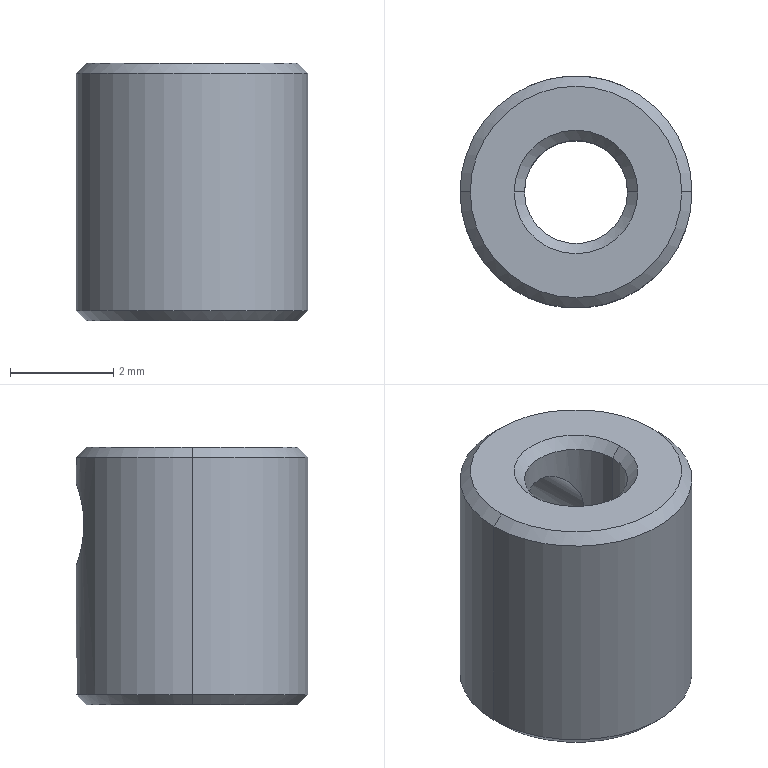Part | SolidWorks | features Chamfer 1, Extrusion 1, HoleWzd 1 | 1 solid | 16 faces | box 4.5 x 4.5 x 5 mm | volume 60.379 mm3 | cone 8 | cylinder 6 | plane 2 | commonest cylinder face diameters 1.6 x2 2 x2 4.5 x2
STEP:
#1=CARTESIAN_POINT('',(0.,2.25,1.8));
#2=VERTEX_POINT('',#1);
#3=CARTESIAN_POINT('',(0.,2.25,0.2));
#4=VERTEX_POINT('',#3);
#5=CARTESIAN_POINT('',(0.,2.25,1.8));
#6=CARTESIAN_POINT('',(-0.105,2.25,1.8));
#7=CARTESIAN_POINT('',(-0.211,2.242,1.779));
#8=CARTESIAN_POINT('',(-0.4042,2.216,1.698));
#9=CARTESIAN_POINT('',(-0.492,2.197,1.639));
#10=CARTESIAN_POINT('',(-0.6398,2.158,1.491));
#11=CARTESIAN_POINT('',(-0.6983,2.139,1.404));
#12=CARTESIAN_POINT('',(-0.779,2.111,1.21));
#13=CARTESIAN_POINT('',(-0.8,2.103,1.105));
#14=CARTESIAN_POINT('',(-0.8,2.103,0.8943));
#15=CARTESIAN_POINT('',(-0.7786,2.111,0.7885));
#16=CARTESIAN_POINT('',(-0.6983,2.139,0.5959));
#17=CARTESIAN_POINT('',(-0.639,2.159,0.5076));
#18=CARTESIAN_POINT('',(-0.4923,2.197,0.361));
#19=CARTESIAN_POINT('',(-0.4046,2.215,0.3019));
#20=CARTESIAN_POINT('',(-0.2107,2.242,0.2211));
#21=CARTESIAN_POINT('',(-0.1066,2.25,0.2));
#22=CARTESIAN_POINT('',(0.,2.25,0.2));
#23=B_SPLINE_CURVE_WITH_KNOTS('',3,(#5,#6,#7,#8,#9,#10,#11,#12,#13,#14,#15,#16,#17,#18,#19,#20,#21,#22),.UNSPECIFIED.,.F.,.F.,(4,2,2,2,2,2,2,2,4),(0.002522,0.002837,0.003152,0.003467,0.003783,0.004098,0.004413,0.004728,0.005043),.UNSPECIFIED.);
#24=EDGE_CURVE('',#2,#4,#23,.T.);
#25=ORIENTED_EDGE('',*,*,#24,.F.);
#26=CARTESIAN_POINT('',(0.,1.,1.8));
#27=VERTEX_POINT('',#26);
#28=CARTESIAN_POINT('',(0.,0.,1.8));
#29=DIRECTION('',(0.,-1.,0.));
#30=VECTOR('',#29,1000.);
#31=LINE('',#28,#30);
#32=EDGE_CURVE('',#2,#27,#31,.T.);
#33=ORIENTED_EDGE('',*,*,#32,.T.);
#34=CARTESIAN_POINT('',(0.,1.,0.2));
#35=VERTEX_POINT('',#34);
#36=CARTESIAN_POINT('',(0.,1.,1.8));
#37=CARTESIAN_POINT('',(-0.1101,1.,1.8));
#38=CARTESIAN_POINT('',(-0.2209,0.9807,1.776));
#39=CARTESIAN_POINT('',(-0.4161,0.9151,1.692));
#40=CARTESIAN_POINT('',(-0.5007,0.8698,1.632));
#41=CARTESIAN_POINT('',(-0.6401,0.7729,1.49));
#42=CARTESIAN_POINT('',(-0.6961,0.7204,1.407));
#43=CARTESIAN_POINT('',(-0.7755,0.6341,1.221));
#44=CARTESIAN_POINT('',(-0.7999,0.6001,1.112));
#45=CARTESIAN_POINT('',(-0.8001,0.5999,0.8891));
#46=CARTESIAN_POINT('',(-0.7764,0.6331,0.7814));
#47=CARTESIAN_POINT('',(-0.6962,0.7203,0.5928));
#48=CARTESIAN_POINT('',(-0.641,0.7723,0.511));
#49=CARTESIAN_POINT('',(-0.5007,0.8698,0.3681));
#50=CARTESIAN_POINT('',(-0.4177,0.9144,0.3094));
#51=CARTESIAN_POINT('',(-0.2225,0.9804,0.2242));
#52=CARTESIAN_POINT('',(-0.1119,1.,0.2));
#53=CARTESIAN_POINT('',(0.,1.,0.2));
#54=B_SPLINE_CURVE_WITH_KNOTS('',3,(#36,#37,#38,#39,#40,#41,#42,#43,#44,#45,#46,#47,#48,#49,#50,#51,#52,#53),.UNSPECIFIED.,.F.,.F.,(4,2,2,2,2,2,2,2,4),(0.002649,0.002979,0.003309,0.003639,0.003969,0.004299,0.00463,0.00496,0.00529),.UNSPECIFIED.);
#55=EDGE_CURVE('',#27,#35,#54,.T.);
#56=ORIENTED_EDGE('',*,*,#55,.T.);
#57=CARTESIAN_POINT('',(0.,0.,0.2));
#58=DIRECTION('',(0.,-1.,0.));
#59=VECTOR('',#58,1000.);
#60=LINE('',#57,#59);
#61=EDGE_CURVE('',#4,#35,#60,.T.);
#62=ORIENTED_EDGE('',*,*,#61,.F.);
#63=EDGE_LOOP('',(#25,#33,#56,#62));
#64=FACE_OUTER_BOUND('',#63,.T.);
#65=CARTESIAN_POINT('',(0.,0.,1.));
#66=DIRECTION('',(0.,-1.,0.));
#67=DIRECTION('',(0.,0.,-1.));
#68=AXIS2_PLACEMENT_3D('',#65,#66,#67);
#69=CYLINDRICAL_SURFACE('',#68,0.8);
#70=ADVANCED_FACE('',(#64),#69,.F.);
#71=CARTESIAN_POINT('',(2.05,0.,2.5));
#72=VERTEX_POINT('',#71);
#73=CARTESIAN_POINT('',(-2.05,0.,2.5));
#74=VERTEX_POINT('',#73);
#75=CARTESIAN_POINT('',(0.,0.,2.5));
#76=DIRECTION('',(0.,0.,1.));
#77=DIRECTION('',(1.,0.,0.));
#78=AXIS2_PLACEMENT_3D('',#75,#76,#77);
#79=CIRCLE('',#78,2.05);
#80=EDGE_CURVE('',#72,#74,#79,.T.);
#81=ORIENTED_EDGE('',*,*,#80,.F.);
#82=CARTESIAN_POINT('',(2.25,0.,2.3));
#83=VERTEX_POINT('',#82);
#84=CARTESIAN_POINT('',(2.05,0.,2.5));
#85=DIRECTION('',(0.7071,0.,-0.7071));
#86=VECTOR('',#85,1000.);
#87=LINE('',#84,#86);
#88=EDGE_CURVE('',#72,#83,#87,.T.);
#89=ORIENTED_EDGE('',*,*,#88,.T.);
#90=CARTESIAN_POINT('',(-2.25,0.,2.3));
#91=VERTEX_POINT('',#90);
#92=CARTESIAN_POINT('',(0.,0.,2.3));
#93=DIRECTION('',(0.,0.,-1.));
#94=DIRECTION('',(1.,0.,0.));
#95=AXIS2_PLACEMENT_3D('',#92,#93,#94);
#96=CIRCLE('',#95,2.25);
#97=EDGE_CURVE('',#91,#83,#96,.T.);
#98=ORIENTED_EDGE('',*,*,#97,.F.);
#99=CARTESIAN_POINT('',(-2.05,0.,2.5));
#100=DIRECTION('',(-0.7071,0.,-0.7071));
#101=VECTOR('',#100,1000.);
#102=LINE('',#99,#101);
#103=EDGE_CURVE('',#74,#91,#102,.T.);
#104=ORIENTED_EDGE('',*,*,#103,.F.);
#105=EDGE_LOOP('',(#81,#89,#98,#104));
#106=FACE_OUTER_BOUND('',#105,.T.);
#107=CARTESIAN_POINT('',(0.,0.,2.5));
#108=DIRECTION('',(0.,0.,-1.));
#109=DIRECTION('',(-1.,0.,0.));
#110=AXIS2_PLACEMENT_3D('',#107,#108,#109);
#111=CONICAL_SURFACE('',#110,2.05,0.7854);
#112=ADVANCED_FACE('',(#106),#111,.T.);
#113=CARTESIAN_POINT('',(-2.05,0.,-2.5));
#114=VERTEX_POINT('',#113);
#115=CARTESIAN_POINT('',(2.05,0.,-2.5));
#116=VERTEX_POINT('',#115);
#117=CARTESIAN_POINT('',(0.,0.,-2.5));
#118=DIRECTION('',(0.,0.,-1.));
#119=DIRECTION('',(1.,0.,0.));
#120=AXIS2_PLACEMENT_3D('',#117,#118,#119);
#121=CIRCLE('',#120,2.05);
#122=EDGE_CURVE('',#114,#116,#121,.T.);
#123=ORIENTED_EDGE('',*,*,#122,.F.);
#124=CARTESIAN_POINT('',(-2.25,0.,-2.3));
#125=VERTEX_POINT('',#124);
#126=CARTESIAN_POINT('',(-2.25,0.,-2.3));
#127=DIRECTION('',(-0.7071,0.,0.7071));
#128=VECTOR('',#127,1000.);
#129=LINE('',#126,#128);
#130=EDGE_CURVE('',#114,#125,#129,.T.);
#131=ORIENTED_EDGE('',*,*,#130,.T.);
#132=CARTESIAN_POINT('',(2.25,0.,-2.3));
#133=VERTEX_POINT('',#132);
#134=CARTESIAN_POINT('',(0.,0.,-2.3));
#135=DIRECTION('',(0.,0.,1.));
#136=DIRECTION('',(1.,0.,0.));
#137=AXIS2_PLACEMENT_3D('',#134,#135,#136);
#138=CIRCLE('',#137,2.25);
#139=EDGE_CURVE('',#133,#125,#138,.T.);
#140=ORIENTED_EDGE('',*,*,#139,.F.);
#141=CARTESIAN_POINT('',(2.25,0.,-2.3));
#142=DIRECTION('',(0.7071,0.,0.7071));
#143=VECTOR('',#142,1000.);
#144=LINE('',#141,#143);
#145=EDGE_CURVE('',#116,#133,#144,.T.);
#146=ORIENTED_EDGE('',*,*,#145,.F.);
#147=EDGE_LOOP('',(#123,#131,#140,#146));
#148=FACE_OUTER_BOUND('',#147,.T.);
#149=CARTESIAN_POINT('',(0.,0.,-2.3));
#150=DIRECTION('',(0.,0.,1.));
#151=DIRECTION('',(1.,0.,0.));
#152=AXIS2_PLACEMENT_3D('',#149,#150,#151);
#153=CONICAL_SURFACE('',#152,2.25,0.7854);
#154=ADVANCED_FACE('',(#148),#153,.T.);
#155=CARTESIAN_POINT('',(-1.,0.,2.3));
#156=VERTEX_POINT('',#155);
#157=CARTESIAN_POINT('',(1.,0.,2.3));
#158=VERTEX_POINT('',#157);
#159=CARTESIAN_POINT('',(0.,0.,2.3));
#160=DIRECTION('',(0.,0.,1.));
#161=DIRECTION('',(1.,0.,0.));
#162=AXIS2_PLACEMENT_3D('',#159,#160,#161);
#163=CIRCLE('',#162,1.);
#164=EDGE_CURVE('',#156,#158,#163,.T.);
#165=ORIENTED_EDGE('',*,*,#164,.F.);
#166=CARTESIAN_POINT('',(-1.2,0.,2.5));
#167=VERTEX_POINT('',#166);
#168=CARTESIAN_POINT('',(-1.,0.,2.3));
#169=DIRECTION('',(-0.7071,0.,0.7071));
#170=VECTOR('',#169,1000.);
#171=LINE('',#168,#170);
#172=EDGE_CURVE('',#156,#167,#171,.T.);
#173=ORIENTED_EDGE('',*,*,#172,.T.);
#174=CARTESIAN_POINT('',(1.2,0.,2.5));
#175=VERTEX_POINT('',#174);
#176=CARTESIAN_POINT('',(0.,0.,2.5));
#177=DIRECTION('',(0.,0.,-1.));
#178=DIRECTION('',(1.,0.,0.));
#179=AXIS2_PLACEMENT_3D('',#176,#177,#178);
#180=CIRCLE('',#179,1.2);
#181=EDGE_CURVE('',#175,#167,#180,.T.);
#182=ORIENTED_EDGE('',*,*,#181,.F.);
#183=CARTESIAN_POINT('',(1.,0.,2.3));
#184=DIRECTION('',(0.7071,0.,0.7071));
#185=VECTOR('',#184,1000.);
#186=LINE('',#183,#185);
#187=EDGE_CURVE('',#158,#175,#186,.T.);
#188=ORIENTED_EDGE('',*,*,#187,.F.);
#189=EDGE_LOOP('',(#165,#173,#182,#188));
#190=FACE_OUTER_BOUND('',#189,.T.);
#191=CARTESIAN_POINT('',(0.,0.,2.3));
#192=DIRECTION('',(0.,0.,1.));
#193=DIRECTION('',(1.,0.,0.));
#194=AXIS2_PLACEMENT_3D('',#191,#192,#193);
#195=CONICAL_SURFACE('',#194,1.,0.7854);
#196=ADVANCED_FACE('',(#190),#195,.F.);
#197=CARTESIAN_POINT('',(1.,0.,-2.3));
#198=VERTEX_POINT('',#197);
#199=CARTESIAN_POINT('',(-1.,0.,-2.3));
#200=VERTEX_POINT('',#199);
#201=CARTESIAN_POINT('',(0.,0.,-2.3));
#202=DIRECTION('',(0.,0.,-1.));
#203=DIRECTION('',(1.,0.,0.));
#204=AXIS2_PLACEMENT_3D('',#201,#202,#203);
#205=CIRCLE('',#204,1.);
#206=EDGE_CURVE('',#198,#200,#205,.T.);
#207=ORIENTED_EDGE('',*,*,#206,.F.);
#208=CARTESIAN_POINT('',(1.2,0.,-2.5));
#209=VERTEX_POINT('',#208);
#210=CARTESIAN_POINT('',(1.2,0.,-2.5));
#211=DIRECTION('',(0.7071,0.,-0.7071));
#212=VECTOR('',#211,1000.);
#213=LINE('',#210,#212);
#214=EDGE_CURVE('',#198,#209,#213,.T.);
#215=ORIENTED_EDGE('',*,*,#214,.T.);
#216=CARTESIAN_POINT('',(-1.2,0.,-2.5));
#217=VERTEX_POINT('',#216);
#218=CARTESIAN_POINT('',(0.,0.,-2.5));
#219=DIRECTION('',(0.,0.,1.));
#220=DIRECTION('',(1.,0.,0.));
#221=AXIS2_PLACEMENT_3D('',#218,#219,#220);
#222=CIRCLE('',#221,1.2);
#223=EDGE_CURVE('',#217,#209,#222,.T.);
#224=ORIENTED_EDGE('',*,*,#223,.F.);
#225=CARTESIAN_POINT('',(-1.2,0.,-2.5));
#226=DIRECTION('',(-0.7071,0.,-0.7071));
#227=VECTOR('',#226,1000.);
#228=LINE('',#225,#227);
#229=EDGE_CURVE('',#200,#217,#228,.T.);
#230=ORIENTED_EDGE('',*,*,#229,.F.);
#231=EDGE_LOOP('',(#207,#215,#224,#230));
#232=FACE_OUTER_BOUND('',#231,.T.);
#233=CARTESIAN_POINT('',(0.,0.,-2.5));
#234=DIRECTION('',(0.,0.,-1.));
#235=DIRECTION('',(-1.,0.,0.));
#236=AXIS2_PLACEMENT_3D('',#233,#234,#235);
#237=CONICAL_SURFACE('',#236,1.2,0.7854);
#238=ADVANCED_FACE('',(#232),#237,.F.);
#239=ORIENTED_EDGE('',*,*,#164,.T.);
#240=CARTESIAN_POINT('',(1.,0.,2.5));
#241=DIRECTION('',(0.,0.,-1.));
#242=VECTOR('',#241,1000.);
#243=LINE('',#240,#242);
#244=EDGE_CURVE('',#158,#198,#243,.T.);
#245=ORIENTED_EDGE('',*,*,#244,.T.);
#246=ORIENTED_EDGE('',*,*,#206,.T.);
#247=CARTESIAN_POINT('',(-1.,0.,2.5));
#248=DIRECTION('',(0.,0.,-1.));
#249=VECTOR('',#248,1000.);
#250=LINE('',#247,#249);
#251=EDGE_CURVE('',#156,#200,#250,.T.);
#252=ORIENTED_EDGE('',*,*,#251,.F.);
#253=EDGE_LOOP('',(#239,#245,#246,#252));
#254=FACE_OUTER_BOUND('',#253,.T.);
#255=CARTESIAN_POINT('',(0.,0.,2.5));
#256=DIRECTION('',(0.,0.,-1.));
#257=DIRECTION('',(-1.,0.,0.));
#258=AXIS2_PLACEMENT_3D('',#255,#256,#257);
#259=CYLINDRICAL_SURFACE('',#258,1.);
#260=ADVANCED_FACE('',(#254),#259,.F.);
#261=CARTESIAN_POINT('',(0.,2.25,0.2));
#262=CARTESIAN_POINT('',(0.1067,2.25,0.2));
#263=CARTESIAN_POINT('',(0.2112,2.242,0.2213));
#264=CARTESIAN_POINT('',(0.4047,2.215,0.302));
#265=CARTESIAN_POINT('',(0.4928,2.197,0.3614));
#266=CARTESIAN_POINT('',(0.6391,2.159,0.5078));
#267=CARTESIAN_POINT('',(0.6984,2.139,0.5963));
#268=CARTESIAN_POINT('',(0.7785,2.111,0.7884));
#269=CARTESIAN_POINT('',(0.7999,2.103,0.8942));
#270=CARTESIAN_POINT('',(0.8001,2.103,1.105));
#271=CARTESIAN_POINT('',(0.7791,2.111,1.21));
#272=CARTESIAN_POINT('',(0.698,2.139,1.405));
#273=CARTESIAN_POINT('',(0.639,2.159,1.492));
#274=CARTESIAN_POINT('',(0.4919,2.197,1.639));
#275=CARTESIAN_POINT('',(0.4037,2.216,1.699));
#276=CARTESIAN_POINT('',(0.2111,2.242,1.779));
#277=CARTESIAN_POINT('',(0.1051,2.25,1.8));
#278=CARTESIAN_POINT('',(0.,2.25,1.8));
#279=B_SPLINE_CURVE_WITH_KNOTS('',3,(#261,#262,#263,#264,#265,#266,#267,#268,#269,#270,#271,#272,#273,#274,#275,#276,#277,#278),.UNSPECIFIED.,.F.,.F.,(4,2,2,2,2,2,2,2,4),(0.,0.0003152,0.0006305,0.0009457,0.001261,0.001576,0.001891,0.002207,0.002522),.UNSPECIFIED.);
#280=EDGE_CURVE('',#4,#2,#279,.T.);
#281=ORIENTED_EDGE('',*,*,#280,.T.);
#282=ORIENTED_EDGE('',*,*,#24,.T.);
#283=EDGE_LOOP('',(#281,#282));
#284=FACE_BOUND('',#283,.T.);
#285=ORIENTED_EDGE('',*,*,#97,.T.);
#286=CARTESIAN_POINT('',(2.25,0.,2.5));
#287=DIRECTION('',(0.,0.,-1.));
#288=VECTOR('',#287,1000.);
#289=LINE('',#286,#288);
#290=EDGE_CURVE('',#83,#133,#289,.T.);
#291=ORIENTED_EDGE('',*,*,#290,.T.);
#292=ORIENTED_EDGE('',*,*,#139,.T.);
#293=CARTESIAN_POINT('',(-2.25,0.,2.5));
#294=DIRECTION('',(0.,0.,-1.));
#295=VECTOR('',#294,1000.);
#296=LINE('',#293,#295);
#297=EDGE_CURVE('',#91,#125,#296,.T.);
#298=ORIENTED_EDGE('',*,*,#297,.F.);
#299=EDGE_LOOP('',(#285,#291,#292,#298));
#300=FACE_OUTER_BOUND('',#299,.T.);
#301=CARTESIAN_POINT('',(0.,0.,2.5));
#302=DIRECTION('',(0.,0.,-1.));
#303=DIRECTION('',(-1.,0.,0.));
#304=AXIS2_PLACEMENT_3D('',#301,#302,#303);
#305=CYLINDRICAL_SURFACE('',#304,2.25);
#306=ADVANCED_FACE('',(#284,#300),#305,.T.);
#307=ORIENTED_EDGE('',*,*,#181,.T.);
#308=CARTESIAN_POINT('',(0.,0.,2.5));
#309=DIRECTION('',(0.,0.,-1.));
#310=DIRECTION('',(1.,0.,0.));
#311=AXIS2_PLACEMENT_3D('',#308,#309,#310);
#312=CIRCLE('',#311,1.2);
#313=EDGE_CURVE('',#167,#175,#312,.T.);
#314=ORIENTED_EDGE('',*,*,#313,.T.);
#315=EDGE_LOOP('',(#307,#314));
#316=FACE_BOUND('',#315,.T.);
#317=CARTESIAN_POINT('',(0.,0.,2.5));
#318=DIRECTION('',(0.,0.,1.));
#319=DIRECTION('',(1.,0.,0.));
#320=AXIS2_PLACEMENT_3D('',#317,#318,#319);
#321=CIRCLE('',#320,2.05);
#322=EDGE_CURVE('',#74,#72,#321,.T.);
#323=ORIENTED_EDGE('',*,*,#322,.T.);
#324=ORIENTED_EDGE('',*,*,#80,.T.);
#325=EDGE_LOOP('',(#323,#324));
#326=FACE_OUTER_BOUND('',#325,.T.);
#327=CARTESIAN_POINT('',(0.,0.,2.5));
#328=DIRECTION('',(0.,0.,1.));
#329=DIRECTION('',(1.,0.,0.));
#330=AXIS2_PLACEMENT_3D('',#327,#328,#329);
#331=PLANE('',#330);
#332=ADVANCED_FACE('',(#316,#326),#331,.T.);
#333=ORIENTED_EDGE('',*,*,#223,.T.);
#334=CARTESIAN_POINT('',(0.,0.,-2.5));
#335=DIRECTION('',(0.,0.,1.));
#336=DIRECTION('',(1.,0.,0.));
#337=AXIS2_PLACEMENT_3D('',#334,#335,#336);
#338=CIRCLE('',#337,1.2);
#339=EDGE_CURVE('',#209,#217,#338,.T.);
#340=ORIENTED_EDGE('',*,*,#339,.T.);
#341=EDGE_LOOP('',(#333,#340));
#342=FACE_BOUND('',#341,.T.);
#343=CARTESIAN_POINT('',(0.,0.,-2.5));
#344=DIRECTION('',(0.,0.,-1.));
#345=DIRECTION('',(1.,0.,0.));
#346=AXIS2_PLACEMENT_3D('',#343,#344,#345);
#347=CIRCLE('',#346,2.05);
#348=EDGE_CURVE('',#116,#114,#347,.T.);
#349=ORIENTED_EDGE('',*,*,#348,.T.);
#350=ORIENTED_EDGE('',*,*,#122,.T.);
#351=EDGE_LOOP('',(#349,#350));
#352=FACE_OUTER_BOUND('',#351,.T.);
#353=CARTESIAN_POINT('',(0.,0.,-2.5));
#354=DIRECTION('',(0.,0.,1.));
#355=DIRECTION('',(1.,0.,0.));
#356=AXIS2_PLACEMENT_3D('',#353,#354,#355);
#357=PLANE('',#356);
#358=ADVANCED_FACE('',(#342,#352),#357,.F.);
#359=ORIENTED_EDGE('',*,*,#290,.F.);
#360=CARTESIAN_POINT('',(0.,0.,2.3));
#361=DIRECTION('',(0.,0.,-1.));
#362=DIRECTION('',(1.,0.,0.));
#363=AXIS2_PLACEMENT_3D('',#360,#361,#362);
#364=CIRCLE('',#363,2.25);
#365=EDGE_CURVE('',#83,#91,#364,.T.);
#366=ORIENTED_EDGE('',*,*,#365,.T.);
#367=ORIENTED_EDGE('',*,*,#297,.T.);
#368=CARTESIAN_POINT('',(0.,0.,-2.3));
#369=DIRECTION('',(0.,0.,1.));
#370=DIRECTION('',(1.,0.,0.));
#371=AXIS2_PLACEMENT_3D('',#368,#369,#370);
#372=CIRCLE('',#371,2.25);
#373=EDGE_CURVE('',#125,#133,#372,.T.);
#374=ORIENTED_EDGE('',*,*,#373,.T.);
#375=EDGE_LOOP('',(#359,#366,#367,#374));
#376=FACE_OUTER_BOUND('',#375,.T.);
#377=CARTESIAN_POINT('',(0.,0.,2.5));
#378=DIRECTION('',(0.,0.,-1.));
#379=DIRECTION('',(-1.,0.,0.));
#380=AXIS2_PLACEMENT_3D('',#377,#378,#379);
#381=CYLINDRICAL_SURFACE('',#380,2.25);
#382=ADVANCED_FACE('',(#376),#381,.T.);
#383=ORIENTED_EDGE('',*,*,#244,.F.);
#384=CARTESIAN_POINT('',(0.,0.,2.3));
#385=DIRECTION('',(0.,0.,1.));
#386=DIRECTION('',(1.,0.,0.));
#387=AXIS2_PLACEMENT_3D('',#384,#385,#386);
#388=CIRCLE('',#387,1.);
#389=EDGE_CURVE('',#158,#156,#388,.T.);
#390=ORIENTED_EDGE('',*,*,#389,.T.);
#391=ORIENTED_EDGE('',*,*,#251,.T.);
#392=CARTESIAN_POINT('',(0.,0.,-2.3));
#393=DIRECTION('',(0.,0.,-1.));
#394=DIRECTION('',(1.,0.,0.));
#395=AXIS2_PLACEMENT_3D('',#392,#393,#394);
#396=CIRCLE('',#395,1.);
#397=EDGE_CURVE('',#200,#198,#396,.T.);
#398=ORIENTED_EDGE('',*,*,#397,.T.);
#399=EDGE_LOOP('',(#383,#390,#391,#398));
#400=FACE_OUTER_BOUND('',#399,.T.);
#401=CARTESIAN_POINT('',(0.,1.,0.2));
#402=CARTESIAN_POINT('',(0.1122,1.,0.2));
#403=CARTESIAN_POINT('',(0.2216,0.9805,0.2241));
#404=CARTESIAN_POINT('',(0.4157,0.9152,0.3084));
#405=CARTESIAN_POINT('',(0.5007,0.8697,0.3682));
#406=CARTESIAN_POINT('',(0.64,0.773,0.5099));
#407=CARTESIAN_POINT('',(0.696,0.7204,0.5927));
#408=CARTESIAN_POINT('',(0.7758,0.6338,0.7797));
#409=CARTESIAN_POINT('',(0.8,0.6,0.8895));
#410=CARTESIAN_POINT('',(0.8,0.6,1.056));
#411=CARTESIAN_POINT('',(0.794,0.6081,1.111));
#412=CARTESIAN_POINT('',(0.772,0.6359,1.217));
#413=CARTESIAN_POINT('',(0.7561,0.6551,1.266));
#414=CARTESIAN_POINT('',(0.6956,0.7209,1.408));
#415=CARTESIAN_POINT('',(0.6404,0.7728,1.49));
#416=CARTESIAN_POINT('',(0.4999,0.8703,1.633));
#417=CARTESIAN_POINT('',(0.4164,0.915,1.691));
#418=CARTESIAN_POINT('',(0.221,0.9807,1.776));
#419=CARTESIAN_POINT('',(0.1105,1.,1.8));
#420=CARTESIAN_POINT('',(0.,1.,1.8));
#421=B_SPLINE_CURVE_WITH_KNOTS('',3,(#401,#402,#403,#404,#405,#406,#407,#408,#409,#410,#411,#412,#413,#414,#415,#416,#417,#418,#419,#420),.UNSPECIFIED.,.F.,.F.,(4,2,2,2,2,2,2,2,2,4),(0.,0.0003311,0.0006623,0.0009934,0.001325,0.00149,0.001656,0.001987,0.002318,0.002649),.UNSPECIFIED.);
#422=EDGE_CURVE('',#35,#27,#421,.T.);
#423=ORIENTED_EDGE('',*,*,#422,.F.);
#424=ORIENTED_EDGE('',*,*,#55,.F.);
#425=EDGE_LOOP('',(#423,#424));
#426=FACE_BOUND('',#425,.T.);
#427=CARTESIAN_POINT('',(0.,0.,2.5));
#428=DIRECTION('',(0.,0.,-1.));
#429=DIRECTION('',(-1.,0.,0.));
#430=AXIS2_PLACEMENT_3D('',#427,#428,#429);
#431=CYLINDRICAL_SURFACE('',#430,1.);
#432=ADVANCED_FACE('',(#400,#426),#431,.F.);
#433=ORIENTED_EDGE('',*,*,#214,.F.);
#434=ORIENTED_EDGE('',*,*,#397,.F.);
#435=ORIENTED_EDGE('',*,*,#229,.T.);
#436=ORIENTED_EDGE('',*,*,#339,.F.);
#437=EDGE_LOOP('',(#433,#434,#435,#436));
#438=FACE_OUTER_BOUND('',#437,.T.);
#439=CARTESIAN_POINT('',(0.,0.,-2.5));
#440=DIRECTION('',(0.,0.,-1.));
#441=DIRECTION('',(-1.,0.,0.));
#442=AXIS2_PLACEMENT_3D('',#439,#440,#441);
#443=CONICAL_SURFACE('',#442,1.2,0.7854);
#444=ADVANCED_FACE('',(#438),#443,.F.);
#445=ORIENTED_EDGE('',*,*,#172,.F.);
#446=ORIENTED_EDGE('',*,*,#389,.F.);
#447=ORIENTED_EDGE('',*,*,#187,.T.);
#448=ORIENTED_EDGE('',*,*,#313,.F.);
#449=EDGE_LOOP('',(#445,#446,#447,#448));
#450=FACE_OUTER_BOUND('',#449,.T.);
#451=CARTESIAN_POINT('',(0.,0.,2.3));
#452=DIRECTION('',(0.,0.,1.));
#453=DIRECTION('',(1.,0.,0.));
#454=AXIS2_PLACEMENT_3D('',#451,#452,#453);
#455=CONICAL_SURFACE('',#454,1.,0.7854);
#456=ADVANCED_FACE('',(#450),#455,.F.);
#457=ORIENTED_EDGE('',*,*,#130,.F.);
#458=ORIENTED_EDGE('',*,*,#348,.F.);
#459=ORIENTED_EDGE('',*,*,#145,.T.);
#460=ORIENTED_EDGE('',*,*,#373,.F.);
#461=EDGE_LOOP('',(#457,#458,#459,#460));
#462=FACE_OUTER_BOUND('',#461,.T.);
#463=CARTESIAN_POINT('',(0.,0.,-2.3));
#464=DIRECTION('',(0.,0.,1.));
#465=DIRECTION('',(1.,0.,0.));
#466=AXIS2_PLACEMENT_3D('',#463,#464,#465);
#467=CONICAL_SURFACE('',#466,2.25,0.7854);
#468=ADVANCED_FACE('',(#462),#467,.T.);
#469=ORIENTED_EDGE('',*,*,#88,.F.);
#470=ORIENTED_EDGE('',*,*,#322,.F.);
#471=ORIENTED_EDGE('',*,*,#103,.T.);
#472=ORIENTED_EDGE('',*,*,#365,.F.);
#473=EDGE_LOOP('',(#469,#470,#471,#472));
#474=FACE_OUTER_BOUND('',#473,.T.);
#475=CARTESIAN_POINT('',(0.,0.,2.5));
#476=DIRECTION('',(0.,0.,-1.));
#477=DIRECTION('',(-1.,0.,0.));
#478=AXIS2_PLACEMENT_3D('',#475,#476,#477);
#479=CONICAL_SURFACE('',#478,2.05,0.7854);
#480=ADVANCED_FACE('',(#474),#479,.T.);
#481=ORIENTED_EDGE('',*,*,#32,.F.);
#482=ORIENTED_EDGE('',*,*,#280,.F.);
#483=ORIENTED_EDGE('',*,*,#61,.T.);
#484=ORIENTED_EDGE('',*,*,#422,.T.);
#485=EDGE_LOOP('',(#481,#482,#483,#484));
#486=FACE_OUTER_BOUND('',#485,.T.);
#487=CARTESIAN_POINT('',(0.,0.,1.));
#488=DIRECTION('',(0.,-1.,0.));
#489=DIRECTION('',(0.,0.,-1.));
#490=AXIS2_PLACEMENT_3D('',#487,#488,#489);
#491=CYLINDRICAL_SURFACE('',#490,0.8);
#492=ADVANCED_FACE('',(#486),#491,.F.);
#493=CLOSED_SHELL('',(#70,#112,#154,#196,#238,#260,#306,#332,#358,#382,#432,#444,#456,#468,#480,#492));
#494=MANIFOLD_SOLID_BREP('',#493);
#495=CARTESIAN_POINT('',(0.,0.,0.));
#496=DIRECTION('',(0.,0.,1.));
#497=DIRECTION('',(1.,0.,0.));
#498=AXIS2_PLACEMENT_3D('',#495,#496,#497);
#499=(LENGTH_UNIT()NAMED_UNIT(*)SI_UNIT(.MILLI.,.METRE.));
#500=UNCERTAINTY_MEASURE_WITH_UNIT(LENGTH_MEASURE(0.00001),#499,'','');
#501=(NAMED_UNIT(*)PLANE_ANGLE_UNIT()SI_UNIT($,.RADIAN.));
#502=(NAMED_UNIT(*)SI_UNIT($,.STERADIAN.)SOLID_ANGLE_UNIT());
#503=(GEOMETRIC_REPRESENTATION_CONTEXT(3)GLOBAL_UNCERTAINTY_ASSIGNED_CONTEXT((#500))GLOBAL_UNIT_ASSIGNED_CONTEXT((#499,#501,#502))REPRESENTATION_CONTEXT('',''));
#504=ADVANCED_BREP_SHAPE_REPRESENTATION('',(#494,#498),#503);